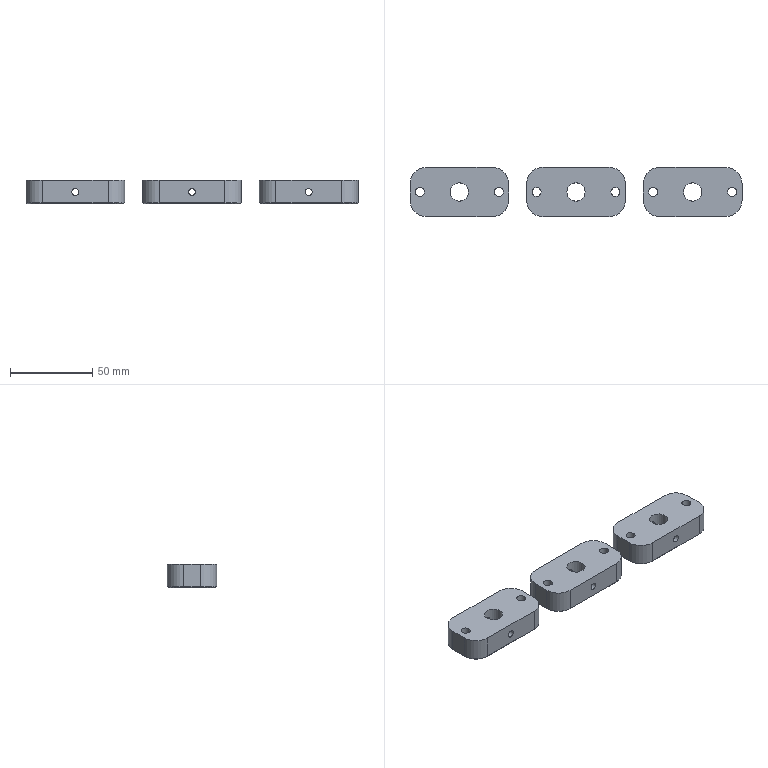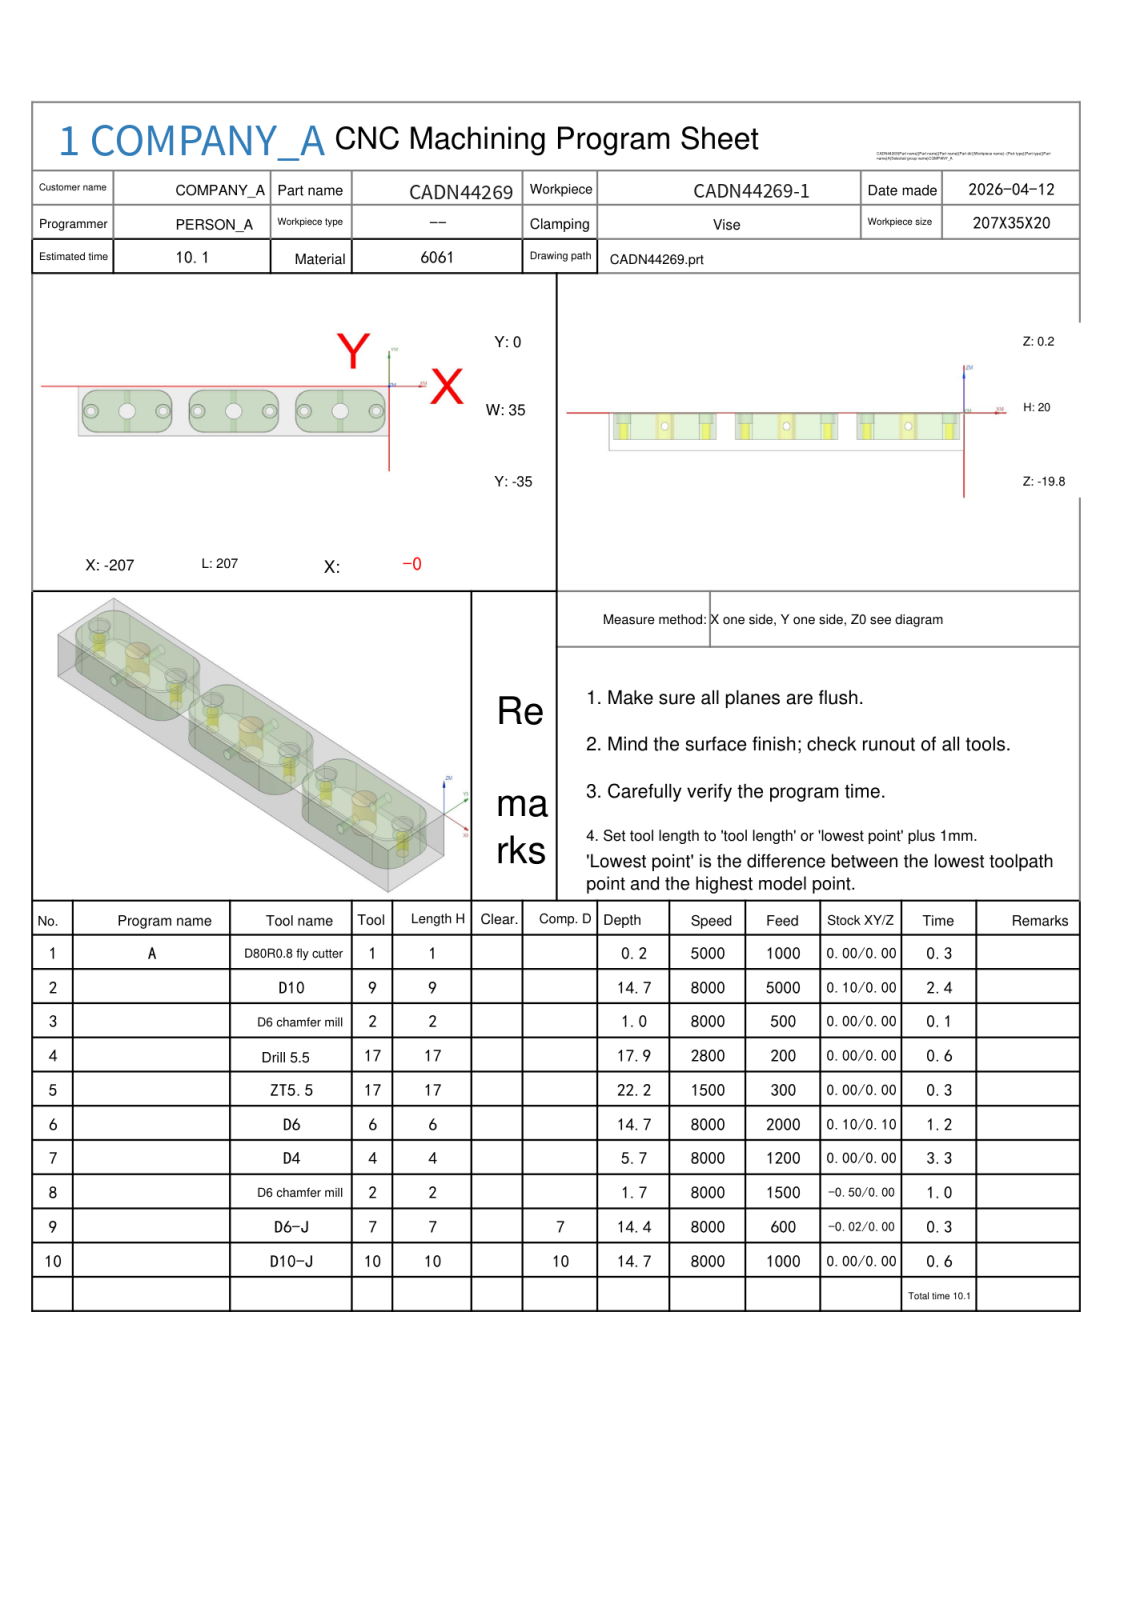NC program | NX | posted by the shop | part box 202 x 30 x 14 mm
Lines 1290 to 2337 of 2337:
N7 T04 M06
(D4  D=4. R=0. H=04 ce=0.10 di=0.00)
G00 G90 G54 X-198.5 Y-17.5 M03 S8000
G43 H04 Z20.
M08
Z1.
G03 X-197.9 Y-18.1 I.6 J0.0 F1200.
X-197.3 Y-17.5 I0.0 J.6
X-197.3 Y-17.5 Z.7 I-1.2 J0.0
X-197.3 Y-17.5 Z.4 I-1.2 J0.0
X-197.3 Y-17.5 Z.1 I-1.2 J0.0
X-197.3 Y-17.5 Z-.2 I-1.2 J0.0
X-197.3 Y-17.5 Z-.5 I-1.2 J0.0
X-197.3 Y-17.5 Z-.8 I-1.2 J0.0
X-197.3 Y-17.5 Z-1.1 I-1.2 J0.0
X-197.3 Y-17.5 Z-1.4 I-1.2 J0.0
X-197.3 Y-17.5 Z-1.7 I-1.2 J0.0
X-197.3 Y-17.5 Z-2. I-1.2 J0.0
X-197.3 Y-17.5 Z-2.3 I-1.2 J0.0
X-197.3 Y-17.5 Z-2.6 I-1.2 J0.0
X-197.3 Y-17.5 Z-2.9 I-1.2 J0.0
X-197.3 Y-17.5 Z-3.2 I-1.2 J0.0
X-197.3 Y-17.5 Z-3.5 I-1.2 J0.0
X-197.3 Y-17.5 Z-3.8 I-1.2 J0.0
X-197.3 Y-17.5 Z-4.1 I-1.2 J0.0
X-197.3 Y-17.5 Z-4.4 I-1.2 J0.0
X-197.3 Y-17.5 Z-4.7 I-1.2 J0.0
X-197.3 Y-17.5 Z-5. I-1.2 J0.0
X-197.3 Y-17.5 Z-5.3 I-1.2 J0.0
X-199.1 Y-18.539 Z-5.5 I-1.2 J0.0
X-198.5 Y-18.7 I.6 J1.039
X-197.3 Y-17.5 I0.0 J1.2
X-198.5 Y-16.3 I-1.2 J0.0
X-199.7 Y-17.5 I0.0 J-1.2
X-199.1 Y-18.539 I1.2 J0.0
X-198.8 Y-18.62 I.3 J.52
X-198.2 Y-18.02 I0.0 J.6
X-198.5 Y-17.5 I-.6 J0.0
G00 Z1.
G03 X-197.3 Y-18.7 I1.2 J0.0
X-196.1 Y-17.5 I0.0 J1.2
X-196.1 Y-17.5 Z.7 I-2.4 J0.0
X-196.1 Y-17.5 Z.4 I-2.4 J0.0
X-196.1 Y-17.5 Z.1 I-2.4 J0.0
X-196.1 Y-17.5 Z-.2 I-2.4 J0.0
X-196.1 Y-17.5 Z-.5 I-2.4 J0.0
X-196.1 Y-17.5 Z-.8 I-2.4 J0.0
X-196.1 Y-17.5 Z-1.1 I-2.4 J0.0
X-196.1 Y-17.5 Z-1.4 I-2.4 J0.0
X-196.1 Y-17.5 Z-1.7 I-2.4 J0.0
X-196.1 Y-17.5 Z-2. I-2.4 J0.0
X-196.1 Y-17.5 Z-2.3 I-2.4 J0.0
X-196.1 Y-17.5 Z-2.6 I-2.4 J0.0
X-196.1 Y-17.5 Z-2.9 I-2.4 J0.0
X-196.1 Y-17.5 Z-3.2 I-2.4 J0.0
X-196.1 Y-17.5 Z-3.5 I-2.4 J0.0
X-196.1 Y-17.5 Z-3.8 I-2.4 J0.0
X-196.1 Y-17.5 Z-4.1 I-2.4 J0.0
X-196.1 Y-17.5 Z-4.4 I-2.4 J0.0
X-196.1 Y-17.5 Z-4.7 I-2.4 J0.0
X-196.1 Y-17.5 Z-5. I-2.4 J0.0
X-196.1 Y-17.5 Z-5.3 I-2.4 J0.0
X-199.7 Y-19.578 Z-5.5 I-2.4 J0.0
X-198.5 Y-19.9 I1.2 J2.078
X-196.1 Y-17.5 I0.0 J2.4
X-198.5 Y-15.1 I-2.4 J0.0
X-200.9 Y-17.5 I0.0 J-2.4
X-199.7 Y-19.578 I2.4 J0.0
X-199.1 Y-19.739 I.6 J1.039
X-197.9 Y-18.539 I0.0 J1.2
X-198.5 Y-17.5 I-1.2 J0.0
G00 Z20.
X-150.5
Z1.
G03 X-149.9 Y-18.1 I.6 J0.0
X-149.3 Y-17.5 I0.0 J.6
X-149.3 Y-17.5 Z.7 I-1.2 J0.0
X-149.3 Y-17.5 Z.4 I-1.2 J0.0
X-149.3 Y-17.5 Z.1 I-1.2 J0.0
X-149.3 Y-17.5 Z-.2 I-1.2 J0.0
X-149.3 Y-17.5 Z-.5 I-1.2 J0.0
X-149.3 Y-17.5 Z-.8 I-1.2 J0.0
X-149.3 Y-17.5 Z-1.1 I-1.2 J0.0
X-149.3 Y-17.5 Z-1.4 I-1.2 J0.0
X-149.3 Y-17.5 Z-1.7 I-1.2 J0.0
X-149.3 Y-17.5 Z-2. I-1.2 J0.0
X-149.3 Y-17.5 Z-2.3 I-1.2 J0.0
X-149.3 Y-17.5 Z-2.6 I-1.2 J0.0
X-149.3 Y-17.5 Z-2.9 I-1.2 J0.0
X-149.3 Y-17.5 Z-3.2 I-1.2 J0.0
X-149.3 Y-17.5 Z-3.5 I-1.2 J0.0
X-149.3 Y-17.5 Z-3.8 I-1.2 J0.0
X-149.3 Y-17.5 Z-4.1 I-1.2 J0.0
X-149.3 Y-17.5 Z-4.4 I-1.2 J0.0
X-149.3 Y-17.5 Z-4.7 I-1.2 J0.0
X-149.3 Y-17.5 Z-5. I-1.2 J0.0
X-149.3 Y-17.5 Z-5.3 I-1.2 J0.0
X-151.1 Y-18.539 Z-5.5 I-1.2 J0.0
X-150.5 Y-18.7 I.6 J1.039
X-149.3 Y-17.5 I0.0 J1.2
X-150.5 Y-16.3 I-1.2 J0.0
X-151.7 Y-17.5 I0.0 J-1.2
X-151.1 Y-18.539 I1.2 J0.0
X-150.8 Y-18.62 I.3 J.52
X-150.2 Y-18.02 I0.0 J.6
X-150.5 Y-17.5 I-.6 J0.0
G00 Z1.
G03 X-149.3 Y-18.7 I1.2 J0.0
X-148.1 Y-17.5 I0.0 J1.2
X-148.1 Y-17.5 Z.7 I-2.4 J0.0
X-148.1 Y-17.5 Z.4 I-2.4 J0.0
X-148.1 Y-17.5 Z.1 I-2.4 J0.0
X-148.1 Y-17.5 Z-.2 I-2.4 J0.0
X-148.1 Y-17.5 Z-.5 I-2.4 J0.0
X-148.1 Y-17.5 Z-.8 I-2.4 J0.0
X-148.1 Y-17.5 Z-1.1 I-2.4 J0.0
X-148.1 Y-17.5 Z-1.4 I-2.4 J0.0
X-148.1 Y-17.5 Z-1.7 I-2.4 J0.0
X-148.1 Y-17.5 Z-2. I-2.4 J0.0
X-148.1 Y-17.5 Z-2.3 I-2.4 J0.0
X-148.1 Y-17.5 Z-2.6 I-2.4 J0.0
X-148.1 Y-17.5 Z-2.9 I-2.4 J0.0
X-148.1 Y-17.5 Z-3.2 I-2.4 J0.0
X-148.1 Y-17.5 Z-3.5 I-2.4 J0.0
X-148.1 Y-17.5 Z-3.8 I-2.4 J0.0
X-148.1 Y-17.5 Z-4.1 I-2.4 J0.0
X-148.1 Y-17.5 Z-4.4 I-2.4 J0.0
X-148.1 Y-17.5 Z-4.7 I-2.4 J0.0
X-148.1 Y-17.5 Z-5. I-2.4 J0.0
X-148.1 Y-17.5 Z-5.3 I-2.4 J0.0
X-151.7 Y-19.578 Z-5.5 I-2.4 J0.0
X-150.5 Y-19.9 I1.2 J2.078
X-148.1 Y-17.5 I0.0 J2.4
X-150.5 Y-15.1 I-2.4 J0.0
X-152.9 Y-17.5 I0.0 J-2.4
X-151.7 Y-19.578 I2.4 J0.0
X-151.1 Y-19.739 I.6 J1.039
X-149.9 Y-18.539 I0.0 J1.2
X-150.5 Y-17.5 I-1.2 J0.0
G00 Z20.
X-127.5
Z1.
G03 X-126.9 Y-18.1 I.6 J0.0
X-126.3 Y-17.5 I0.0 J.6
X-126.3 Y-17.5 Z.7 I-1.2 J0.0
X-126.3 Y-17.5 Z.4 I-1.2 J0.0
X-126.3 Y-17.5 Z.1 I-1.2 J0.0
X-126.3 Y-17.5 Z-.2 I-1.2 J0.0
X-126.3 Y-17.5 Z-.5 I-1.2 J0.0
X-126.3 Y-17.5 Z-.8 I-1.2 J0.0
X-126.3 Y-17.5 Z-1.1 I-1.2 J0.0
X-126.3 Y-17.5 Z-1.4 I-1.2 J0.0
X-126.3 Y-17.5 Z-1.7 I-1.2 J0.0
X-126.3 Y-17.5 Z-2. I-1.2 J0.0
X-126.3 Y-17.5 Z-2.3 I-1.2 J0.0
X-126.3 Y-17.5 Z-2.6 I-1.2 J0.0
X-126.3 Y-17.5 Z-2.9 I-1.2 J0.0
X-126.3 Y-17.5 Z-3.2 I-1.2 J0.0
X-126.3 Y-17.5 Z-3.5 I-1.2 J0.0
X-126.3 Y-17.5 Z-3.8 I-1.2 J0.0
X-126.3 Y-17.5 Z-4.1 I-1.2 J0.0
X-126.3 Y-17.5 Z-4.4 I-1.2 J0.0
X-126.3 Y-17.5 Z-4.7 I-1.2 J0.0
X-126.3 Y-17.5 Z-5. I-1.2 J0.0
X-126.3 Y-17.5 Z-5.3 I-1.2 J0.0
X-128.1 Y-18.539 Z-5.5 I-1.2 J0.0
X-127.5 Y-18.7 I.6 J1.039
X-126.3 Y-17.5 I0.0 J1.2
X-127.5 Y-16.3 I-1.2 J0.0
X-128.7 Y-17.5 I0.0 J-1.2
X-128.1 Y-18.539 I1.2 J0.0
X-127.8 Y-18.62 I.3 J.52
X-127.2 Y-18.02 I0.0 J.6
X-127.5 Y-17.5 I-.6 J0.0
G00 Z1.
G03 X-126.3 Y-18.7 I1.2 J0.0
X-125.1 Y-17.5 I0.0 J1.2
X-125.1 Y-17.5 Z.7 I-2.4 J0.0
X-125.1 Y-17.5 Z.4 I-2.4 J0.0
X-125.1 Y-17.5 Z.1 I-2.4 J0.0
X-125.1 Y-17.5 Z-.2 I-2.4 J0.0
X-125.1 Y-17.5 Z-.5 I-2.4 J0.0
X-125.1 Y-17.5 Z-.8 I-2.4 J0.0
X-125.1 Y-17.5 Z-1.1 I-2.4 J0.0
X-125.1 Y-17.5 Z-1.4 I-2.4 J0.0
X-125.1 Y-17.5 Z-1.7 I-2.4 J0.0
X-125.1 Y-17.5 Z-2. I-2.4 J0.0
X-125.1 Y-17.5 Z-2.3 I-2.4 J0.0
X-125.1 Y-17.5 Z-2.6 I-2.4 J0.0
X-125.1 Y-17.5 Z-2.9 I-2.4 J0.0
X-125.1 Y-17.5 Z-3.2 I-2.4 J0.0
X-125.1 Y-17.5 Z-3.5 I-2.4 J0.0
X-125.1 Y-17.5 Z-3.8 I-2.4 J0.0
X-125.1 Y-17.5 Z-4.1 I-2.4 J0.0
X-125.1 Y-17.5 Z-4.4 I-2.4 J0.0
X-125.1 Y-17.5 Z-4.7 I-2.4 J0.0
X-125.1 Y-17.5 Z-5. I-2.4 J0.0
X-125.1 Y-17.5 Z-5.3 I-2.4 J0.0
X-128.7 Y-19.578 Z-5.5 I-2.4 J0.0
X-127.5 Y-19.9 I1.2 J2.078
X-125.1 Y-17.5 I0.0 J2.4
X-127.5 Y-15.1 I-2.4 J0.0
X-129.9 Y-17.5 I0.0 J-2.4
X-128.7 Y-19.578 I2.4 J0.0
X-128.1 Y-19.739 I.6 J1.039
X-126.9 Y-18.539 I0.0 J1.2
X-127.5 Y-17.5 I-1.2 J0.0
G00 Z20.
X-79.5
Z1.
G03 X-78.9 Y-18.1 I.6 J0.0
X-78.3 Y-17.5 I0.0 J.6
X-78.3 Y-17.5 Z.7 I-1.2 J0.0
X-78.3 Y-17.5 Z.4 I-1.2 J0.0
X-78.3 Y-17.5 Z.1 I-1.2 J0.0
X-78.3 Y-17.5 Z-.2 I-1.2 J0.0
X-78.3 Y-17.5 Z-.5 I-1.2 J0.0
X-78.3 Y-17.5 Z-.8 I-1.2 J0.0
X-78.3 Y-17.5 Z-1.1 I-1.2 J0.0
X-78.3 Y-17.5 Z-1.4 I-1.2 J0.0
X-78.3 Y-17.5 Z-1.7 I-1.2 J0.0
X-78.3 Y-17.5 Z-2. I-1.2 J0.0
X-78.3 Y-17.5 Z-2.3 I-1.2 J0.0
X-78.3 Y-17.5 Z-2.6 I-1.2 J0.0
X-78.3 Y-17.5 Z-2.9 I-1.2 J0.0
X-78.3 Y-17.5 Z-3.2 I-1.2 J0.0
X-78.3 Y-17.5 Z-3.5 I-1.2 J0.0
X-78.3 Y-17.5 Z-3.8 I-1.2 J0.0
X-78.3 Y-17.5 Z-4.1 I-1.2 J0.0
X-78.3 Y-17.5 Z-4.4 I-1.2 J0.0
X-78.3 Y-17.5 Z-4.7 I-1.2 J0.0
X-78.3 Y-17.5 Z-5. I-1.2 J0.0
X-78.3 Y-17.5 Z-5.3 I-1.2 J0.0
X-80.1 Y-18.539 Z-5.5 I-1.2 J0.0
X-79.5 Y-18.7 I.6 J1.039
X-78.3 Y-17.5 I0.0 J1.2
X-79.5 Y-16.3 I-1.2 J0.0
X-80.7 Y-17.5 I0.0 J-1.2
X-80.1 Y-18.539 I1.2 J0.0
X-79.8 Y-18.62 I.3 J.52
X-79.2 Y-18.02 I0.0 J.6
X-79.5 Y-17.5 I-.6 J0.0
G00 Z1.
G03 X-78.3 Y-18.7 I1.2 J0.0
X-77.1 Y-17.5 I0.0 J1.2
X-77.1 Y-17.5 Z.7 I-2.4 J0.0
X-77.1 Y-17.5 Z.4 I-2.4 J0.0
X-77.1 Y-17.5 Z.1 I-2.4 J0.0
X-77.1 Y-17.5 Z-.2 I-2.4 J0.0
X-77.1 Y-17.5 Z-.5 I-2.4 J0.0
X-77.1 Y-17.5 Z-.8 I-2.4 J0.0
X-77.1 Y-17.5 Z-1.1 I-2.4 J0.0
X-77.1 Y-17.5 Z-1.4 I-2.4 J0.0
X-77.1 Y-17.5 Z-1.7 I-2.4 J0.0
X-77.1 Y-17.5 Z-2. I-2.4 J0.0
X-77.1 Y-17.5 Z-2.3 I-2.4 J0.0
X-77.1 Y-17.5 Z-2.6 I-2.4 J0.0
X-77.1 Y-17.5 Z-2.9 I-2.4 J0.0
X-77.1 Y-17.5 Z-3.2 I-2.4 J0.0
X-77.1 Y-17.5 Z-3.5 I-2.4 J0.0
X-77.1 Y-17.5 Z-3.8 I-2.4 J0.0
X-77.1 Y-17.5 Z-4.1 I-2.4 J0.0
X-77.1 Y-17.5 Z-4.4 I-2.4 J0.0
X-77.1 Y-17.5 Z-4.7 I-2.4 J0.0
X-77.1 Y-17.5 Z-5. I-2.4 J0.0
X-77.1 Y-17.5 Z-5.3 I-2.4 J0.0
X-80.7 Y-19.578 Z-5.5 I-2.4 J0.0
X-79.5 Y-19.9 I1.2 J2.078
X-77.1 Y-17.5 I0.0 J2.4
X-79.5 Y-15.1 I-2.4 J0.0
X-81.9 Y-17.5 I0.0 J-2.4
X-80.7 Y-19.578 I2.4 J0.0
X-80.1 Y-19.739 I.6 J1.039
X-78.9 Y-18.539 I0.0 J1.2
X-79.5 Y-17.5 I-1.2 J0.0
G00 Z20.
X-56.5
Z1.
G03 X-55.9 Y-18.1 I.6 J0.0
X-55.3 Y-17.5 I0.0 J.6
X-55.3 Y-17.5 Z.7 I-1.2 J0.0
X-55.3 Y-17.5 Z.4 I-1.2 J0.0
X-55.3 Y-17.5 Z.1 I-1.2 J0.0
X-55.3 Y-17.5 Z-.2 I-1.2 J0.0
X-55.3 Y-17.5 Z-.5 I-1.2 J0.0
X-55.3 Y-17.5 Z-.8 I-1.2 J0.0
X-55.3 Y-17.5 Z-1.1 I-1.2 J0.0
X-55.3 Y-17.5 Z-1.4 I-1.2 J0.0
X-55.3 Y-17.5 Z-1.7 I-1.2 J0.0
X-55.3 Y-17.5 Z-2. I-1.2 J0.0
X-55.3 Y-17.5 Z-2.3 I-1.2 J0.0
X-55.3 Y-17.5 Z-2.6 I-1.2 J0.0
X-55.3 Y-17.5 Z-2.9 I-1.2 J0.0
X-55.3 Y-17.5 Z-3.2 I-1.2 J0.0
X-55.3 Y-17.5 Z-3.5 I-1.2 J0.0
X-55.3 Y-17.5 Z-3.8 I-1.2 J0.0
X-55.3 Y-17.5 Z-4.1 I-1.2 J0.0
X-55.3 Y-17.5 Z-4.4 I-1.2 J0.0
X-55.3 Y-17.5 Z-4.7 I-1.2 J0.0
X-55.3 Y-17.5 Z-5. I-1.2 J0.0
X-55.3 Y-17.5 Z-5.3 I-1.2 J0.0
X-57.1 Y-18.539 Z-5.5 I-1.2 J0.0
X-56.5 Y-18.7 I.6 J1.039
X-55.3 Y-17.5 I0.0 J1.2
X-56.5 Y-16.3 I-1.2 J0.0
X-57.7 Y-17.5 I0.0 J-1.2
X-57.1 Y-18.539 I1.2 J0.0
X-56.8 Y-18.62 I.3 J.52
X-56.2 Y-18.02 I0.0 J.6
X-56.5 Y-17.5 I-.6 J0.0
G00 Z1.
G03 X-55.3 Y-18.7 I1.2 J0.0
X-54.1 Y-17.5 I0.0 J1.2
X-54.1 Y-17.5 Z.7 I-2.4 J0.0
X-54.1 Y-17.5 Z.4 I-2.4 J0.0
X-54.1 Y-17.5 Z.1 I-2.4 J0.0
X-54.1 Y-17.5 Z-.2 I-2.4 J0.0
X-54.1 Y-17.5 Z-.5 I-2.4 J0.0
X-54.1 Y-17.5 Z-.8 I-2.4 J0.0
X-54.1 Y-17.5 Z-1.1 I-2.4 J0.0
X-54.1 Y-17.5 Z-1.4 I-2.4 J0.0
X-54.1 Y-17.5 Z-1.7 I-2.4 J0.0
X-54.1 Y-17.5 Z-2. I-2.4 J0.0
X-54.1 Y-17.5 Z-2.3 I-2.4 J0.0
X-54.1 Y-17.5 Z-2.6 I-2.4 J0.0
X-54.1 Y-17.5 Z-2.9 I-2.4 J0.0
X-54.1 Y-17.5 Z-3.2 I-2.4 J0.0
X-54.1 Y-17.5 Z-3.5 I-2.4 J0.0
X-54.1 Y-17.5 Z-3.8 I-2.4 J0.0
X-54.1 Y-17.5 Z-4.1 I-2.4 J0.0
X-54.1 Y-17.5 Z-4.4 I-2.4 J0.0
X-54.1 Y-17.5 Z-4.7 I-2.4 J0.0
X-54.1 Y-17.5 Z-5. I-2.4 J0.0
X-54.1 Y-17.5 Z-5.3 I-2.4 J0.0
X-57.7 Y-19.578 Z-5.5 I-2.4 J0.0
X-56.5 Y-19.9 I1.2 J2.078
X-54.1 Y-17.5 I0.0 J2.4
X-56.5 Y-15.1 I-2.4 J0.0
X-58.9 Y-17.5 I0.0 J-2.4
X-57.7 Y-19.578 I2.4 J0.0
X-57.1 Y-19.739 I.6 J1.039
X-55.9 Y-18.539 I0.0 J1.2
X-56.5 Y-17.5 I-1.2 J0.0
G00 Z20.
X-8.5
Z1.
G03 X-7.9 Y-18.1 I.6 J0.0
X-7.3 Y-17.5 I0.0 J.6
X-7.3 Y-17.5 Z.7 I-1.2 J0.0
X-7.3 Y-17.5 Z.4 I-1.2 J0.0
X-7.3 Y-17.5 Z.1 I-1.2 J0.0
X-7.3 Y-17.5 Z-.2 I-1.2 J0.0
X-7.3 Y-17.5 Z-.5 I-1.2 J0.0
X-7.3 Y-17.5 Z-.8 I-1.2 J0.0
X-7.3 Y-17.5 Z-1.1 I-1.2 J0.0
X-7.3 Y-17.5 Z-1.4 I-1.2 J0.0
X-7.3 Y-17.5 Z-1.7 I-1.2 J0.0
X-7.3 Y-17.5 Z-2. I-1.2 J0.0
X-7.3 Y-17.5 Z-2.3 I-1.2 J0.0
X-7.3 Y-17.5 Z-2.6 I-1.2 J0.0
X-7.3 Y-17.5 Z-2.9 I-1.2 J0.0
X-7.3 Y-17.5 Z-3.2 I-1.2 J0.0
X-7.3 Y-17.5 Z-3.5 I-1.2 J0.0
X-7.3 Y-17.5 Z-3.8 I-1.2 J0.0
X-7.3 Y-17.5 Z-4.1 I-1.2 J0.0
X-7.3 Y-17.5 Z-4.4 I-1.2 J0.0
X-7.3 Y-17.5 Z-4.7 I-1.2 J0.0
X-7.3 Y-17.5 Z-5. I-1.2 J0.0
X-7.3 Y-17.5 Z-5.3 I-1.2 J0.0
X-9.1 Y-18.539 Z-5.5 I-1.2 J0.0
X-8.5 Y-18.7 I.6 J1.039
X-7.3 Y-17.5 I0.0 J1.2
X-8.5 Y-16.3 I-1.2 J0.0
X-9.7 Y-17.5 I0.0 J-1.2
X-9.1 Y-18.539 I1.2 J0.0
X-8.8 Y-18.62 I.3 J.52
X-8.2 Y-18.02 I0.0 J.6
X-8.5 Y-17.5 I-.6 J0.0
G00 Z1.
G03 X-7.3 Y-18.7 I1.2 J0.0
X-6.1 Y-17.5 I0.0 J1.2
X-6.1 Y-17.5 Z.7 I-2.4 J0.0
X-6.1 Y-17.5 Z.4 I-2.4 J0.0
X-6.1 Y-17.5 Z.1 I-2.4 J0.0
X-6.1 Y-17.5 Z-.2 I-2.4 J0.0
X-6.1 Y-17.5 Z-.5 I-2.4 J0.0
X-6.1 Y-17.5 Z-.8 I-2.4 J0.0
X-6.1 Y-17.5 Z-1.1 I-2.4 J0.0
X-6.1 Y-17.5 Z-1.4 I-2.4 J0.0
X-6.1 Y-17.5 Z-1.7 I-2.4 J0.0
X-6.1 Y-17.5 Z-2. I-2.4 J0.0
X-6.1 Y-17.5 Z-2.3 I-2.4 J0.0
X-6.1 Y-17.5 Z-2.6 I-2.4 J0.0
X-6.1 Y-17.5 Z-2.9 I-2.4 J0.0
X-6.1 Y-17.5 Z-3.2 I-2.4 J0.0
X-6.1 Y-17.5 Z-3.5 I-2.4 J0.0
X-6.1 Y-17.5 Z-3.8 I-2.4 J0.0
X-6.1 Y-17.5 Z-4.1 I-2.4 J0.0
X-6.1 Y-17.5 Z-4.4 I-2.4 J0.0
X-6.1 Y-17.5 Z-4.7 I-2.4 J0.0
X-6.1 Y-17.5 Z-5. I-2.4 J0.0
X-6.1 Y-17.5 Z-5.3 I-2.4 J0.0
X-9.7 Y-19.578 Z-5.5 I-2.4 J0.0
X-8.5 Y-19.9 I1.2 J2.078
X-6.1 Y-17.5 I0.0 J2.4
X-8.5 Y-15.1 I-2.4 J0.0
X-10.9 Y-17.5 I0.0 J-2.4
X-9.7 Y-19.578 I2.4 J0.0
X-9.1 Y-19.739 I.6 J1.039
X-7.9 Y-18.539 I0.0 J1.2
X-8.5 Y-17.5 I-1.2 J0.0
G00 Z20.
G00 G90 X-198.5 Y-17.5 M03 S8000
Z20.
Z1.
G41 D04
G01 X-198.468 Y-17.697 F500.
G03 X-197.242 Y-18.742 I1.226 J.197
X-196. Y-17.5 I0.0 J1.242
X-196. Y-17.5 Z-4. I-2.5 J0.0
X-199.273 Y-15.122 Z-5.5 I-2.5 J0.0
X-201. Y-17.5 I.773 J-2.378
X-198.5 Y-20. I2.5 J0.0
X-196. Y-17.5 I0.0 J2.5
X-198.5 Y-15. I-2.5 J0.0
X-199.273 Y-15.122 I0.0 J-2.5
X-200.131 Y-16.304 I.384 J-1.181
X-198.889 Y-17.546 I1.242 J0.0
G01 X-198.698 Y-17.531
G40 X-198.5 Y-17.5
G00 Z20.
X-150.5
Z1.
G41 D04
G01 X-150.468 Y-17.697
G03 X-149.242 Y-18.742 I1.226 J.197
X-148. Y-17.5 I0.0 J1.242
X-148. Y-17.5 Z-4. I-2.5 J0.0
X-151.273 Y-15.122 Z-5.5 I-2.5 J0.0
X-153. Y-17.5 I.773 J-2.378
X-150.5 Y-20. I2.5 J0.0
X-148. Y-17.5 I0.0 J2.5
X-150.5 Y-15. I-2.5 J0.0
X-151.273 Y-15.122 I0.0 J-2.5
X-152.131 Y-16.304 I.384 J-1.181
X-150.889 Y-17.546 I1.242 J0.0
G01 X-150.698 Y-17.531
G40 X-150.5 Y-17.5
G00 Z20.
X-127.5
Z1.
G41 D04
G01 X-127.468 Y-17.697
G03 X-126.242 Y-18.742 I1.226 J.197
X-125. Y-17.5 I0.0 J1.242
X-125. Y-17.5 Z-4. I-2.5 J0.0
X-128.273 Y-15.122 Z-5.5 I-2.5 J0.0
X-130. Y-17.5 I.773 J-2.378
X-127.5 Y-20. I2.5 J0.0
X-125. Y-17.5 I0.0 J2.5
X-127.5 Y-15. I-2.5 J0.0
X-128.273 Y-15.122 I0.0 J-2.5
X-129.131 Y-16.304 I.384 J-1.181
X-127.889 Y-17.546 I1.242 J0.0
G01 X-127.698 Y-17.531
G40 X-127.5 Y-17.5
G00 Z20.
X-79.5
Z1.
G41 D04
G01 X-79.468 Y-17.697
G03 X-78.242 Y-18.742 I1.226 J.197
X-77. Y-17.5 I0.0 J1.242
X-77. Y-17.5 Z-4. I-2.5 J0.0
X-80.273 Y-15.122 Z-5.5 I-2.5 J0.0
X-82. Y-17.5 I.773 J-2.378
X-79.5 Y-20. I2.5 J0.0
X-77. Y-17.5 I0.0 J2.5
X-79.5 Y-15. I-2.5 J0.0
X-80.273 Y-15.122 I0.0 J-2.5
X-81.131 Y-16.304 I.384 J-1.181
X-79.889 Y-17.546 I1.242 J0.0
G01 X-79.698 Y-17.531
G40 X-79.5 Y-17.5
G00 Z20.
X-56.5
Z1.
G41 D04
G01 X-56.468 Y-17.697
G03 X-55.242 Y-18.742 I1.226 J.197
X-54. Y-17.5 I0.0 J1.242
X-54. Y-17.5 Z-4. I-2.5 J0.0
X-57.273 Y-15.122 Z-5.5 I-2.5 J0.0
X-59. Y-17.5 I.773 J-2.378
X-56.5 Y-20. I2.5 J0.0
X-54. Y-17.5 I0.0 J2.5
X-56.5 Y-15. I-2.5 J0.0
X-57.273 Y-15.122 I0.0 J-2.5
X-58.131 Y-16.304 I.384 J-1.181
X-56.889 Y-17.546 I1.242 J0.0
G01 X-56.698 Y-17.531
G40 X-56.5 Y-17.5
G00 Z20.
X-8.5
Z1.
G41 D04
G01 X-8.468 Y-17.697
G03 X-7.242 Y-18.742 I1.226 J.197
X-6. Y-17.5 I0.0 J1.242
X-6. Y-17.5 Z-4. I-2.5 J0.0
X-9.273 Y-15.122 Z-5.5 I-2.5 J0.0
X-11. Y-17.5 I.773 J-2.378
X-8.5 Y-20. I2.5 J0.0
X-6. Y-17.5 I0.0 J2.5
X-8.5 Y-15. I-2.5 J0.0
X-9.273 Y-15.122 I0.0 J-2.5
X-10.131 Y-16.304 I.384 J-1.181
X-8.889 Y-17.546 I1.242 J0.0
G01 X-8.698 Y-17.531
G40 X-8.5 Y-17.5
G00 Z20.
G91 G28 Z0.0
M05
M09
G91 G28 Z0.0
M01
N8 T02 M06
(D6 chamfer mill  D=6. R=0. H=02 ce=-0.50 di=0.00)
G00 G90 G54 X-4.998 Y-17.491 M03 S8000
G43 H02 Z20.
M08
Z2.5
G01 X-5.019 Y-17.109 Z2.361 F500.
X-5.084 Y-16.724 Z2.219
X-5.192 Y-16.347 Z2.076
X-5.341 Y-15.986 Z1.934
X-5.53 Y-15.643 Z1.791
X-5.755 Y-15.323 Z1.649
X-6.015 Y-15.031 Z1.507
X-6.306 Y-14.769 Z1.364
X-6.624 Y-14.541 Z1.222
X-6.876 Y-14.396 Z1.116
X-7.232 Y-14.235 Z.974
X-7.604 Y-14.114 Z.831
X-7.987 Y-14.035 Z.689
X-8.377 Y-13.999 Z.547
X-8.768 Y-14.007 Z.404
X-9.156 Y-14.059 Z.262
X-9.535 Y-14.154 Z.119
X-9.902 Y-14.29 Z-.023
X-10.252 Y-14.466 Z-.166
X-10.579 Y-14.681 Z-.308
X-10.88 Y-14.93 Z-.45
X-11.152 Y-15.212 Z-.593
X-11.391 Y-15.522 Z-.735
X-11.593 Y-15.856 Z-.878
X-11.757 Y-16.212 Z-1.02
X-11.881 Y-16.583 Z-1.162
X-11.962 Y-16.966 Z-1.305
X-12. Y-17.355 Z-1.447
Y-17.5 Z-1.5
G03 X-8.5 Y-21. I3.5 J0.0
X-5. Y-17.5 I0.0 J3.5
X-8.5 Y-14. I-3.5 J0.0
X-12. Y-17.5 I0.0 J-3.5
X-11.964 Y-17.998 I3.5 J0.0
G01 Z1.
G00 Z20.
X-52.998 Y-17.491
Z2.5
G01 X-53.019 Y-17.109 Z2.361
X-53.084 Y-16.724 Z2.219
X-53.192 Y-16.347 Z2.076
X-53.341 Y-15.986 Z1.934
X-53.53 Y-15.643 Z1.791
X-53.755 Y-15.323 Z1.649
X-54.015 Y-15.031 Z1.507
X-54.306 Y-14.769 Z1.364
X-54.624 Y-14.541 Z1.222
X-54.876 Y-14.396 Z1.116
X-55.232 Y-14.235 Z.974
X-55.604 Y-14.114 Z.831
X-55.987 Y-14.035 Z.689
X-56.377 Y-13.999 Z.547
X-56.768 Y-14.007 Z.404
X-57.156 Y-14.059 Z.262
X-57.535 Y-14.154 Z.119
X-57.902 Y-14.29 Z-.023
X-58.252 Y-14.466 Z-.166
X-58.579 Y-14.681 Z-.308
X-58.88 Y-14.93 Z-.45
X-59.152 Y-15.212 Z-.593
X-59.391 Y-15.522 Z-.735
X-59.593 Y-15.856 Z-.878
X-59.757 Y-16.212 Z-1.02
X-59.881 Y-16.583 Z-1.162
X-59.962 Y-16.966 Z-1.305
X-60. Y-17.355 Z-1.447
Y-17.5 Z-1.5
G03 X-56.5 Y-21. I3.5 J0.0
X-53. Y-17.5 I0.0 J3.5
X-56.5 Y-14. I-3.5 J0.0
X-60. Y-17.5 I0.0 J-3.5
X-59.964 Y-17.998 I3.5 J0.0
G01 Z1.
G00 Z20.
X-75.998 Y-17.491
Z2.5
G01 X-76.019 Y-17.109 Z2.361
X-76.084 Y-16.724 Z2.219
X-76.192 Y-16.347 Z2.076
X-76.341 Y-15.986 Z1.934
X-76.53 Y-15.643 Z1.791
X-76.755 Y-15.323 Z1.649
X-77.015 Y-15.031 Z1.507
X-77.306 Y-14.769 Z1.364
X-77.624 Y-14.541 Z1.222
X-77.876 Y-14.396 Z1.116
X-78.232 Y-14.235 Z.974
X-78.604 Y-14.114 Z.831
X-78.987 Y-14.035 Z.689
X-79.377 Y-13.999 Z.547
X-79.768 Y-14.007 Z.404
X-80.156 Y-14.059 Z.262
X-80.535 Y-14.154 Z.119
X-80.902 Y-14.29 Z-.023
X-81.252 Y-14.466 Z-.166
X-81.579 Y-14.681 Z-.308
X-81.88 Y-14.93 Z-.45
X-82.152 Y-15.212 Z-.593
X-82.391 Y-15.522 Z-.735
X-82.593 Y-15.856 Z-.878
X-82.757 Y-16.212 Z-1.02
X-82.881 Y-16.583 Z-1.162
X-82.962 Y-16.966 Z-1.305
X-83. Y-17.355 Z-1.447
Y-17.5 Z-1.5
G03 X-79.5 Y-21. I3.5 J0.0
X-76. Y-17.5 I0.0 J3.5
X-79.5 Y-14. I-3.5 J0.0
X-83. Y-17.5 I0.0 J-3.5
X-82.964 Y-17.998 I3.5 J0.0
G01 Z1.
G00 Z20.
X-123.998 Y-17.491
Z2.5
G01 X-124.019 Y-17.109 Z2.361
X-124.084 Y-16.724 Z2.219
X-124.192 Y-16.347 Z2.076
X-124.341 Y-15.986 Z1.934
X-124.53 Y-15.643 Z1.791
X-124.755 Y-15.323 Z1.649
X-125.015 Y-15.031 Z1.507
X-125.306 Y-14.769 Z1.364
X-125.624 Y-14.541 Z1.222
X-125.876 Y-14.396 Z1.116
X-126.232 Y-14.235 Z.974
X-126.604 Y-14.114 Z.831
X-126.987 Y-14.035 Z.689
X-127.377 Y-13.999 Z.547
X-127.768 Y-14.007 Z.404
X-128.156 Y-14.059 Z.262
X-128.535 Y-14.154 Z.119
X-128.902 Y-14.29 Z-.023
X-129.252 Y-14.466 Z-.166
X-129.579 Y-14.681 Z-.308
X-129.88 Y-14.93 Z-.45
X-130.152 Y-15.212 Z-.593
X-130.391 Y-15.522 Z-.735
X-130.593 Y-15.856 Z-.878
X-130.757 Y-16.212 Z-1.02
X-130.881 Y-16.583 Z-1.162
X-130.962 Y-16.966 Z-1.305
X-131. Y-17.355 Z-1.447
Y-17.5 Z-1.5
G03 X-127.5 Y-21. I3.5 J0.0
X-124. Y-17.5 I0.0 J3.5
X-127.5 Y-14. I-3.5 J0.0
X-131. Y-17.5 I0.0 J-3.5
X-130.964 Y-17.998 I3.5 J0.0
G01 Z1.
G00 Z20.
X-146.998 Y-17.491
Z2.5
G01 X-147.019 Y-17.109 Z2.361
X-147.084 Y-16.724 Z2.219
X-147.192 Y-16.347 Z2.076
X-147.341 Y-15.986 Z1.934
X-147.53 Y-15.643 Z1.791
X-147.755 Y-15.323 Z1.649
X-148.015 Y-15.031 Z1.507
X-148.306 Y-14.769 Z1.364
X-148.624 Y-14.541 Z1.222
X-148.876 Y-14.396 Z1.116
X-149.232 Y-14.235 Z.974
X-149.604 Y-14.114 Z.831
X-149.987 Y-14.035 Z.689
X-150.377 Y-13.999 Z.547
X-150.768 Y-14.007 Z.404
X-151.156 Y-14.059 Z.262
X-151.535 Y-14.154 Z.119
X-151.902 Y-14.29 Z-.023
X-152.252 Y-14.466 Z-.166
X-152.579 Y-14.681 Z-.308
X-152.88 Y-14.93 Z-.45
X-153.152 Y-15.212 Z-.593
X-153.391 Y-15.522 Z-.735
X-153.593 Y-15.856 Z-.878
X-153.757 Y-16.212 Z-1.02
X-153.881 Y-16.583 Z-1.162
X-153.962 Y-16.966 Z-1.305
X-154. Y-17.355 Z-1.447
Y-17.5 Z-1.5
G03 X-150.5 Y-21. I3.5 J0.0
X-147. Y-17.5 I0.0 J3.5
X-150.5 Y-14. I-3.5 J0.0
X-154. Y-17.5 I0.0 J-3.5
X-153.964 Y-17.998 I3.5 J0.0
G01 Z1.
G00 Z20.
X-194.998 Y-17.491
Z2.5
G01 X-195.019 Y-17.109 Z2.361
X-195.084 Y-16.724 Z2.219
X-195.192 Y-16.347 Z2.076
X-195.341 Y-15.986 Z1.934
X-195.53 Y-15.643 Z1.791
X-195.755 Y-15.323 Z1.649
X-196.015 Y-15.031 Z1.507
X-196.306 Y-14.769 Z1.364
X-196.624 Y-14.541 Z1.222
X-196.876 Y-14.396 Z1.116
X-197.232 Y-14.235 Z.974
X-197.604 Y-14.114 Z.831
X-197.987 Y-14.035 Z.689
X-198.377 Y-13.999 Z.547
X-198.768 Y-14.007 Z.404
X-199.156 Y-14.059 Z.262
X-199.535 Y-14.154 Z.119
X-199.902 Y-14.29 Z-.023
X-200.252 Y-14.466 Z-.166
X-200.579 Y-14.681 Z-.308
X-200.88 Y-14.93 Z-.45
X-201.152 Y-15.212 Z-.593
X-201.391 Y-15.522 Z-.735
X-201.593 Y-15.856 Z-.878
X-201.757 Y-16.212 Z-1.02
X-201.881 Y-16.583 Z-1.162
X-201.962 Y-16.966 Z-1.305
X-202. Y-17.355 Z-1.447
Y-17.5 Z-1.5
G03 X-198.5 Y-21. I3.5 J0.0
X-195. Y-17.5 I0.0 J3.5
X-198.5 Y-14. I-3.5 J0.0
X-202. Y-17.5 I0.0 J-3.5
X-201.964 Y-17.998 I3.5 J0.0
G01 Z1.
G00 Z20.
G00 G90 X-172.67 Y-20.5 M03 S8000
Z20.
Z-.5
G01 Z-1. F800.
G03 X-169.67 Y-17.5 I0.0 J3.
X-174.5 Y-12.67 I-4.83 J0.0
X-179.33 Y-17.5 I0.0 J-4.83
X-174.5 Y-22.33 I4.83 J0.0
X-169.67 Y-17.5 I0.0 J4.83
X-172.67 Y-14.5 I-3. J0.0
G01 Z-.5
G00 Z20.
X-101.67 Y-20.5
Z-.5
G01 Z-1.
G03 X-98.67 Y-17.5 I0.0 J3.
X-103.5 Y-12.67 I-4.83 J0.0
X-108.33 Y-17.5 I0.0 J-4.83
X-103.5 Y-22.33 I4.83 J0.0
X-98.67 Y-17.5 I0.0 J4.83
X-101.67 Y-14.5 I-3. J0.0
G01 Z-.5
G00 Z20.
X-30.67 Y-20.5
Z-.5
G01 Z-1.
G03 X-27.67 Y-17.5 I0.0 J3.
X-32.5 Y-12.67 I-4.83 J0.0
X-37.33 Y-17.5 I0.0 J-4.83
X-32.5 Y-22.33 I4.83 J0.0
X-27.67 Y-17.5 I0.0 J4.83
X-30.67 Y-14.5 I-3. J0.0
G01 Z-.5
G00 Z20.
G00 G90 X-79.008 Y-33.52 M03 S6500
Z20.
Z.3
G01 Z-1.2 F1500.
G03 X-80.141 Y-32.716 I-1.133 J-.396
X-80.479 Y-32.765 I0.0 J-1.2
G02 X-81.164 Y-32.942 I-3.021 J10.265
X-83.5 Y-33.2 I-2.336 J10.442
G01 X-123.5
G02 X-134.2 Y-22.5 I0.0 J10.7
G01 Y-12.5
G02 X-123.5 Y-1.8 I10.7 J0.0
G01 X-83.5
G02 X-78.509 Y-3.036 I0.0 J-10.7
X-78.221 Y-3.193 I-4.991 J-9.464
G01 X-78.208 Y-3.2
X-78.148 Y-3.235
X-78.004 Y-3.319
G02 X-75.07 Y-5.91 I-5.496 J-9.181
X-72.8 Y-12.5 I-8.43 J-6.59
G01 Y-22.5
G02 X-73.438 Y-26.141 I-10.7 J0.0
X-80.479 Y-32.765 I-10.062 J3.641
X-80.865 Y-32.871 I-3.021 J10.265
G03 X-81.77 Y-34.034 I.295 J-1.163
X-81.746 Y-34.27 I1.2 J0.0
G01 Z.3
G00 X-31.3 Y-34.4
G01 Z-1.2
G03 X-32.5 Y-33.2 I-1.2 J0.0
G01 X-52.5
G02 X-63.2 Y-22.5 I0.0 J10.7
G01 Y-12.5
G02 X-52.5 Y-1.8 I10.7 J0.0
G01 X-12.5
G02 X-1.8 Y-12.5 I0.0 J-10.7
G01 Y-22.5
G02 X-4.33 Y-29.41 I-10.7 J0.0
G01 X-4.433 Y-29.53
G02 X-4.795 Y-29.924 I-8.067 J7.03
X-7.163 Y-31.774 I-7.705 J7.424
X-12.5 Y-33.2 I-5.337 J9.274
G01 X-32.5
X-32.9
G03 X-34.1 Y-34.4 I0.0 J-1.2
G01 Z.3
G00 X-171.848
G01 Z-1.2
G03 X-173.048 Y-33.2 I-1.2 J0.0
G01 X-194.5
G02 X-205.2 Y-22.5 I0.0 J10.7
G01 Y-12.5
G02 X-201.265 Y-4.21 I10.7 J0.0
G01 X-201.118 Y-4.092
X-201.027 Y-4.021
G02 X-194.5 Y-1.8 I6.527 J-8.479
G01 X-154.5
G02 X-143.8 Y-12.5 I0.0 J-10.7
G01 Y-22.5
G02 X-149.863 Y-32.143 I-10.7 J0.0
G01 X-150.024 Y-32.219
G02 X-150.392 Y-32.38 I-4.476 J9.719
G01 X-150.438 Y-32.399
X-150.594 Y-32.462
X-150.625 Y-32.474
G02 X-152.722 Y-33.051 I-3.875 J9.974
X-153.208 Y-33.122 I-1.778 J10.551
X-153.427 Y-33.146 I-1.292 J10.622
X-154.5 Y-33.2 I-1.073 J10.646
G01 X-173.048
X-173.448
G03 X-174.648 Y-34.4 I0.0 J-1.2
G01 Z.3
G00 Z20.
G91 G28 Z0.0
M05
M09
G91 G28 Z0.0
M01
N9 T07 M06
(D6-J  D=6. R=0. H=07 ce=-0.02 di=0.00)
G00 G90 G54 X-173.6 Y-16.317 M03 S8000
G43 H07 Z10.2
M08
Z-5.6
G01 Z-7.1 F600.
G41 D07
Y-15.85
G03 X-174.5 Y-14.95 I-.9 J0.0
X-177.05 Y-17.5 I0.0 J-2.55
X-174.5 Y-20.05 I2.55 J0.0
X-171.95 Y-17.5 I0.0 J2.55
X-174.5 Y-14.95 I-2.55 J0.0
X-174.898 Y-14.981 I0.0 J-2.55
X-175.658 Y-15.87 I.141 J-.889
G01 X-175.647 Y-16.011
X-175.605 Y-16.275
G40 X-175.574 Y-16.472
Z-5.6
G00 X-173.6 Y-16.317
Z-12.7
G01 Z-14.2
G41 D07
Y-15.85
G03 X-174.5 Y-14.95 I-.9 J0.0
X-177.05 Y-17.5 I0.0 J-2.55
X-174.5 Y-20.05 I2.55 J0.0
X-171.95 Y-17.5 I0.0 J2.55
X-174.5 Y-14.95 I-2.55 J0.0
X-174.898 Y-14.981 I0.0 J-2.55
X-175.658 Y-15.87 I.141 J-.889
G01 X-175.647 Y-16.011
X-175.605 Y-16.275
G40 X-175.574 Y-16.472
Z-12.7
G00 Z10.2
X-104.4 Y-18.683
Z-5.6
G01 Z-7.1
G41 D07
Y-19.15
G03 X-103.5 Y-20.05 I.9 J0.0
X-100.95 Y-17.5 I0.0 J2.55
X-103.5 Y-14.95 I-2.55 J0.0
X-106.05 Y-17.5 I0.0 J-2.55
X-103.5 Y-20.05 I2.55 J0.0
X-103.102 Y-20.019 I0.0 J2.55
X-102.342 Y-19.13 I-.141 J.889
G01 X-102.353 Y-18.989
X-102.395 Y-18.725
G40 X-102.426 Y-18.528
Z-5.6
G00 X-104.4 Y-18.683
Z-12.7
G01 Z-14.2
G41 D07
Y-19.15
G03 X-103.5 Y-20.05 I.9 J0.0
X-100.95 Y-17.5 I0.0 J2.55
X-103.5 Y-14.95 I-2.55 J0.0
X-106.05 Y-17.5 I0.0 J-2.55
X-103.5 Y-20.05 I2.55 J0.0
X-103.102 Y-20.019 I0.0 J2.55
X-102.342 Y-19.13 I-.141 J.889
G01 X-102.353 Y-18.989
X-102.395 Y-18.725
G40 X-102.426 Y-18.528
Z-12.7
G00 Z10.2
X-33.4 Y-18.683
Z-5.6
G01 Z-7.1
G41 D07
Y-19.15
G03 X-32.5 Y-20.05 I.9 J0.0
X-29.95 Y-17.5 I0.0 J2.55
X-32.5 Y-14.95 I-2.55 J0.0
X-35.05 Y-17.5 I0.0 J-2.55
X-32.5 Y-20.05 I2.55 J0.0
X-32.102 Y-20.019 I0.0 J2.55
X-31.342 Y-19.13 I-.141 J.889
G01 X-31.353 Y-18.989
X-31.395 Y-18.725
G40 X-31.426 Y-18.528
Z-5.6
G00 X-33.4 Y-18.683
Z-12.7
G01 Z-14.2
G41 D07
Y-19.15
G03 X-32.5 Y-20.05 I.9 J0.0
X-29.95 Y-17.5 I0.0 J2.55
X-32.5 Y-14.95 I-2.55 J0.0
X-35.05 Y-17.5 I0.0 J-2.55
X-32.5 Y-20.05 I2.55 J0.0
X-32.102 Y-20.019 I0.0 J2.55
X-31.342 Y-19.13 I-.141 J.889
G01 X-31.353 Y-18.989
X-31.395 Y-18.725
G40 X-31.426 Y-18.528
Z-12.7
G00 Z10.2
G91 G28 Z0.0
M05
M09
G91 G28 Z0.0
M01
N10 T10 M06
(D10-J  D=10. R=0. H=10 ce=0.00 di=0.00)
G00 G90 G54 X-195.506 Y3.669 M03 S8000
G43 H10 Z20.
M08
Z-14.
G01 Z-14.5 F1000.
G41 D10
X-195.5 Y3.469
G03 X-194.5 Y2.5 I1. J.031
G01 X-154.5
G02 X-139.5 Y-12.5 I0.0 J-15.
G01 Y-22.5
G02 X-154.5 Y-37.5 I-15. J0.0
G01 X-194.5
G02 X-209.5 Y-22.5 I0.0 J15.
G01 Y-12.5
G02 X-194.5 Y2.5 I15. J0.0
G01 X-194.
G03 X-193. Y3.5 I0.0 J1.
G01 G40 Y3.7
Z-14.
G00 Z20.
X-104.5
Z-14.
G01 Z-14.5
G41 D10
Y3.5
G03 X-103.5 Y2.5 I1. J0.0
G01 X-83.5
G02 X-68.5 Y-12.5 I0.0 J-15.
G01 Y-22.5
G02 X-83.5 Y-37.5 I-15. J0.0
G01 X-123.5
G02 X-138.5 Y-22.5 I0.0 J15.
G01 Y-12.5
G02 X-123.5 Y2.5 I15. J0.0
G01 X-103.5
X-103.
G03 X-102. Y3.5 I0.0 J1.
G01 G40 Y3.7
Z-14.
G00 Z20.
X-33.5
Z-14.
G01 Z-14.5
G41 D10
Y3.5
G03 X-32.5 Y2.5 I1. J0.0
G01 X-12.5
G02 X2.5 Y-12.5 I0.0 J-15.
G01 Y-22.5
G02 X-12.5 Y-37.5 I-15. J0.0
G01 X-52.5
G02 X-67.5 Y-22.5 I0.0 J15.
G01 Y-12.5
G02 X-52.5 Y2.5 I15. J0.0
G01 X-32.5
X-32.
G03 X-31. Y3.5 I0.0 J1.
G01 G40 Y3.7
Z-14.
G00 Z20.
M05
M09
G91 G28 Z0.0
G91 G28 Y0.0
M30
%